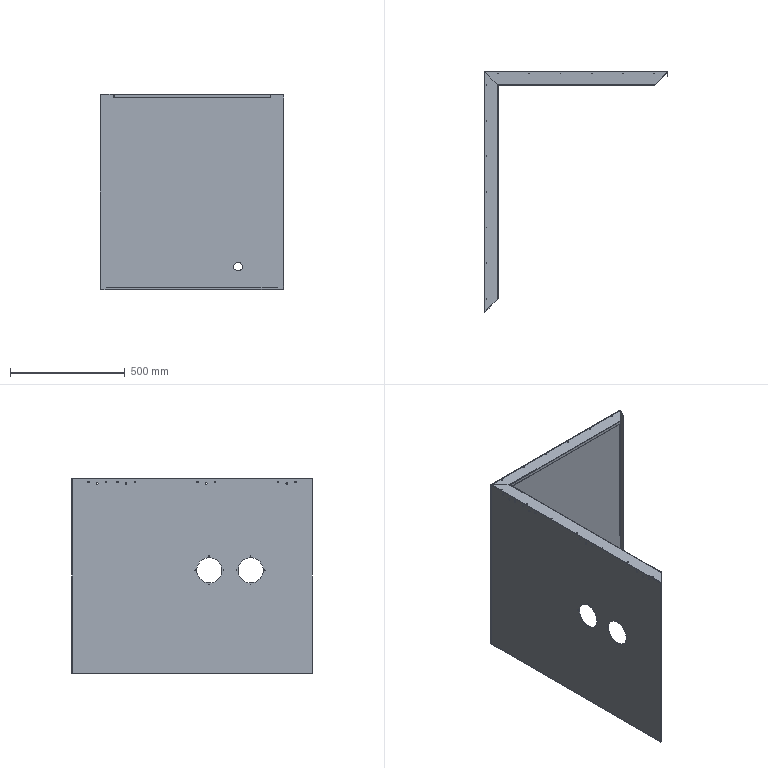Part | STEP file | HESS-408-70-15W-W-3-outer case side panel 3 | 1 solid | 170 faces | box 798.5 x 1049 x 850 mm | volume 2623190 mm3 | cylinder 92 | plane 72 | spline 6 | commonest cylinder face diameters 3.2 x26 3.5 x26 7 x24 0.2 x10 110 x4 38.5 x2